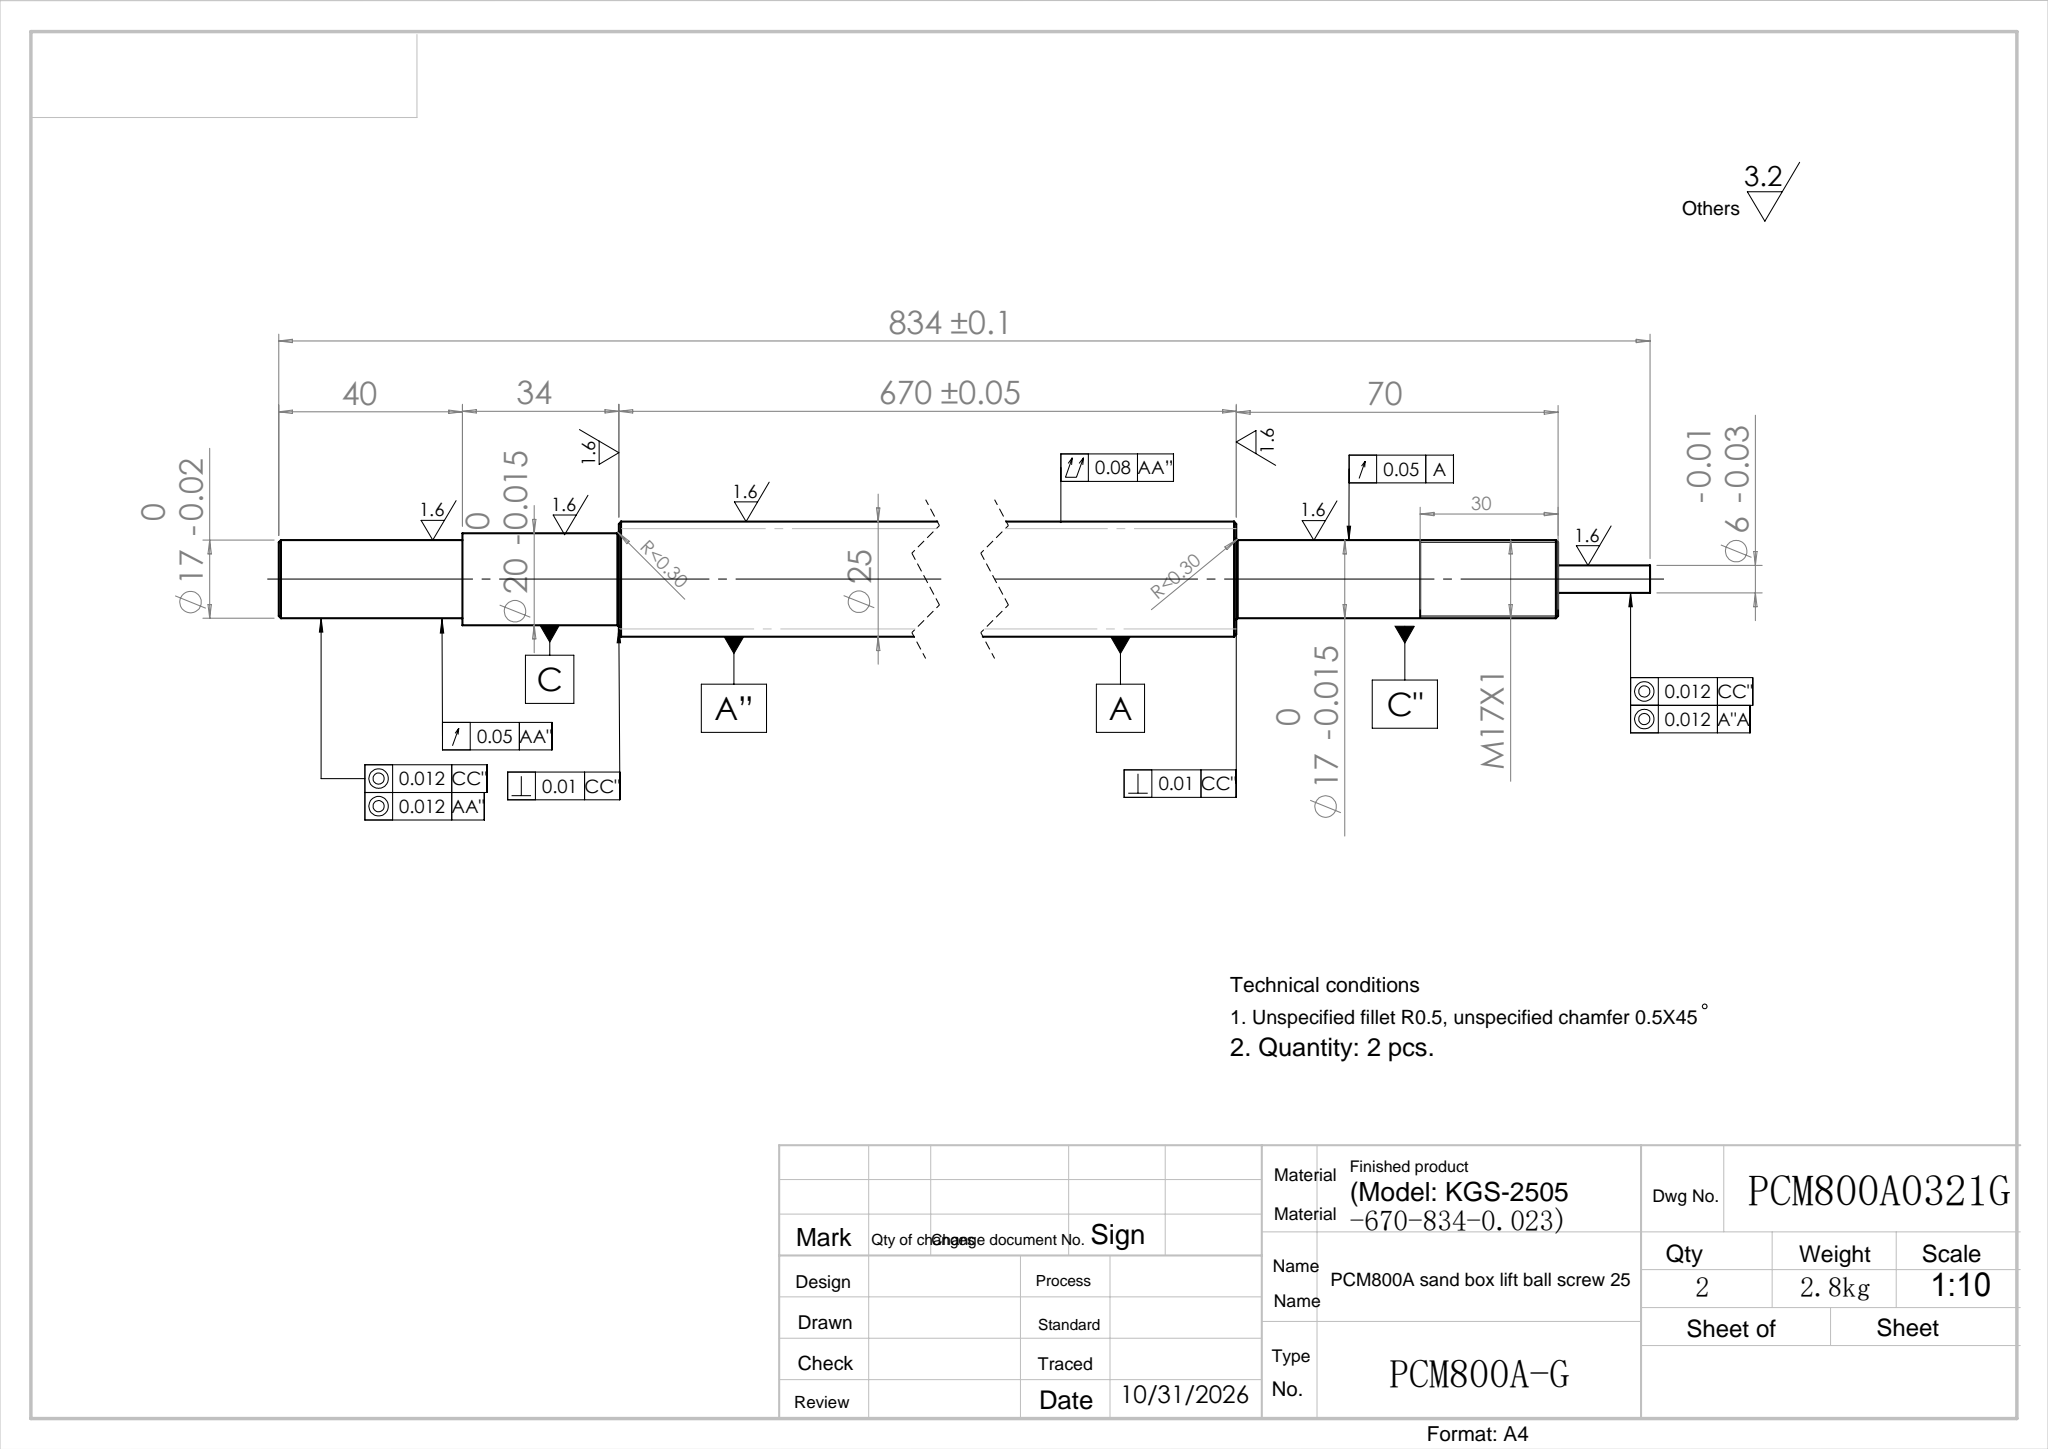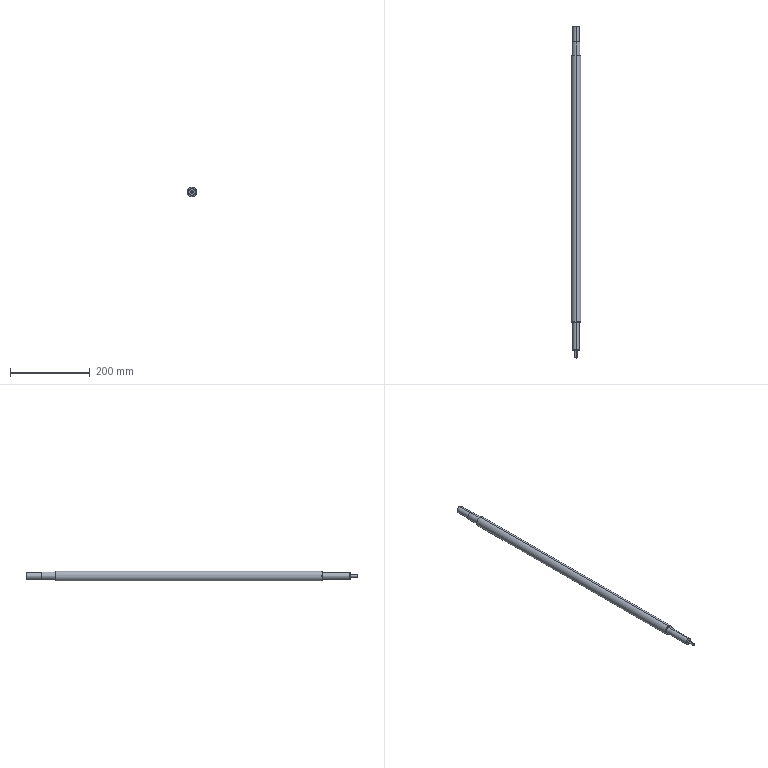Part | SolidWorks | features Boss 4, Fillet 2, Chamfer 1, Extrusion 1 | 1 solid | 28 faces | box 25 x 834 x 25 mm | volume 365070 mm3 | cylinder 10 | cone 8 | plane 6 | torus 4 | commonest cylinder face diameters 17 x4 6 x2 20 x2 25 x2
STEP:
#1=CARTESIAN_POINT('',(0.,-20.,-3.));
#2=VERTEX_POINT('',#1);
#3=CARTESIAN_POINT('',(0.,-20.,3.));
#4=VERTEX_POINT('',#3);
#5=CARTESIAN_POINT('',(0.,-20.,0.));
#6=DIRECTION('',(0.,-1.,0.));
#7=DIRECTION('',(0.,0.,-1.));
#8=AXIS2_PLACEMENT_3D('',#5,#6,#7);
#9=CIRCLE('',#8,3.);
#10=EDGE_CURVE('',#2,#4,#9,.T.);
#11=ORIENTED_EDGE('',*,*,#10,.F.);
#12=CARTESIAN_POINT('',(0.,0.,-3.));
#13=VERTEX_POINT('',#12);
#14=CARTESIAN_POINT('',(0.,-20.,-3.));
#15=DIRECTION('',(0.,1.,0.));
#16=VECTOR('',#15,1000.);
#17=LINE('',#14,#16);
#18=EDGE_CURVE('',#2,#13,#17,.T.);
#19=ORIENTED_EDGE('',*,*,#18,.T.);
#20=CARTESIAN_POINT('',(0.,0.,3.));
#21=VERTEX_POINT('',#20);
#22=CARTESIAN_POINT('',(0.,0.,0.));
#23=DIRECTION('',(0.,-1.,0.));
#24=DIRECTION('',(0.,0.,1.));
#25=AXIS2_PLACEMENT_3D('',#22,#23,#24);
#26=CIRCLE('',#25,3.);
#27=EDGE_CURVE('',#13,#21,#26,.T.);
#28=ORIENTED_EDGE('',*,*,#27,.T.);
#29=CARTESIAN_POINT('',(0.,-20.,3.));
#30=DIRECTION('',(0.,1.,0.));
#31=VECTOR('',#30,1000.);
#32=LINE('',#29,#31);
#33=EDGE_CURVE('',#4,#21,#32,.T.);
#34=ORIENTED_EDGE('',*,*,#33,.F.);
#35=EDGE_LOOP('',(#11,#19,#28,#34));
#36=FACE_OUTER_BOUND('',#35,.T.);
#37=CARTESIAN_POINT('',(0.,-20.,0.));
#38=DIRECTION('',(0.,1.,0.));
#39=DIRECTION('',(0.,0.,1.));
#40=AXIS2_PLACEMENT_3D('',#37,#38,#39);
#41=CYLINDRICAL_SURFACE('',#40,3.);
#42=ADVANCED_FACE('',(#36),#41,.T.);
#43=CARTESIAN_POINT('',(0.,740.3,-10.));
#44=VERTEX_POINT('',#43);
#45=CARTESIAN_POINT('',(0.,740.3,10.));
#46=VERTEX_POINT('',#45);
#47=CARTESIAN_POINT('',(0.,740.3,0.));
#48=DIRECTION('',(0.,1.,0.));
#49=DIRECTION('',(0.,0.,1.));
#50=AXIS2_PLACEMENT_3D('',#47,#48,#49);
#51=CIRCLE('',#50,10.);
#52=EDGE_CURVE('',#44,#46,#51,.T.);
#53=ORIENTED_EDGE('',*,*,#52,.F.);
#54=CARTESIAN_POINT('',(0.,740.,-10.3));
#55=VERTEX_POINT('',#54);
#56=CARTESIAN_POINT('',(0.,740.3,-10.3));
#57=DIRECTION('',(1.,0.,0.));
#58=DIRECTION('',(0.,0.,-1.));
#59=AXIS2_PLACEMENT_3D('',#56,#57,#58);
#60=CIRCLE('',#59,0.3);
#61=EDGE_CURVE('',#44,#55,#60,.T.);
#62=ORIENTED_EDGE('',*,*,#61,.T.);
#63=CARTESIAN_POINT('',(0.,740.,10.3));
#64=VERTEX_POINT('',#63);
#65=CARTESIAN_POINT('',(0.,740.,0.));
#66=DIRECTION('',(0.,-1.,0.));
#67=DIRECTION('',(0.,0.,1.));
#68=AXIS2_PLACEMENT_3D('',#65,#66,#67);
#69=CIRCLE('',#68,10.3);
#70=EDGE_CURVE('',#64,#55,#69,.T.);
#71=ORIENTED_EDGE('',*,*,#70,.F.);
#72=CARTESIAN_POINT('',(0.,740.3,10.3));
#73=DIRECTION('',(-1.,0.,0.));
#74=DIRECTION('',(0.,0.,1.));
#75=AXIS2_PLACEMENT_3D('',#72,#73,#74);
#76=CIRCLE('',#75,0.3);
#77=EDGE_CURVE('',#46,#64,#76,.T.);
#78=ORIENTED_EDGE('',*,*,#77,.F.);
#79=EDGE_LOOP('',(#53,#62,#71,#78));
#80=FACE_OUTER_BOUND('',#79,.T.);
#81=CARTESIAN_POINT('',(0.,740.3,0.));
#82=DIRECTION('',(0.,1.,0.));
#83=DIRECTION('',(0.,0.,1.));
#84=AXIS2_PLACEMENT_3D('',#81,#82,#83);
#85=TOROIDAL_SURFACE('',#84,10.3,0.3);
#86=ADVANCED_FACE('',(#80),#85,.F.);
#87=CARTESIAN_POINT('',(0.,70.,-8.8));
#88=VERTEX_POINT('',#87);
#89=CARTESIAN_POINT('',(0.,70.,8.8));
#90=VERTEX_POINT('',#89);
#91=CARTESIAN_POINT('',(0.,70.,0.));
#92=DIRECTION('',(0.,1.,0.));
#93=DIRECTION('',(0.,0.,1.));
#94=AXIS2_PLACEMENT_3D('',#91,#92,#93);
#95=CIRCLE('',#94,8.8);
#96=EDGE_CURVE('',#88,#90,#95,.T.);
#97=ORIENTED_EDGE('',*,*,#96,.F.);
#98=CARTESIAN_POINT('',(0.,69.7,-8.5));
#99=VERTEX_POINT('',#98);
#100=CARTESIAN_POINT('',(0.,69.7,-8.8));
#101=DIRECTION('',(1.,0.,0.));
#102=DIRECTION('',(0.,0.,-1.));
#103=AXIS2_PLACEMENT_3D('',#100,#101,#102);
#104=CIRCLE('',#103,0.3);
#105=EDGE_CURVE('',#88,#99,#104,.T.);
#106=ORIENTED_EDGE('',*,*,#105,.T.);
#107=CARTESIAN_POINT('',(0.,69.7,8.5));
#108=VERTEX_POINT('',#107);
#109=CARTESIAN_POINT('',(0.,69.7,0.));
#110=DIRECTION('',(0.,-1.,0.));
#111=DIRECTION('',(0.,0.,1.));
#112=AXIS2_PLACEMENT_3D('',#109,#110,#111);
#113=CIRCLE('',#112,8.5);
#114=EDGE_CURVE('',#108,#99,#113,.T.);
#115=ORIENTED_EDGE('',*,*,#114,.F.);
#116=CARTESIAN_POINT('',(0.,69.7,8.8));
#117=DIRECTION('',(-1.,0.,0.));
#118=DIRECTION('',(0.,0.,1.));
#119=AXIS2_PLACEMENT_3D('',#116,#117,#118);
#120=CIRCLE('',#119,0.3);
#121=EDGE_CURVE('',#90,#108,#120,.T.);
#122=ORIENTED_EDGE('',*,*,#121,.F.);
#123=EDGE_LOOP('',(#97,#106,#115,#122));
#124=FACE_OUTER_BOUND('',#123,.T.);
#125=CARTESIAN_POINT('',(0.,69.7,0.));
#126=DIRECTION('',(0.,1.,0.));
#127=DIRECTION('',(0.,0.,1.));
#128=AXIS2_PLACEMENT_3D('',#125,#126,#127);
#129=TOROIDAL_SURFACE('',#128,8.8,0.3);
#130=ADVANCED_FACE('',(#124),#129,.F.);
#131=CARTESIAN_POINT('',(0.,814.,8.));
#132=VERTEX_POINT('',#131);
#133=CARTESIAN_POINT('',(0.,814.,-8.));
#134=VERTEX_POINT('',#133);
#135=CARTESIAN_POINT('',(0.,814.,0.));
#136=DIRECTION('',(0.,1.,0.));
#137=DIRECTION('',(0.,0.,1.));
#138=AXIS2_PLACEMENT_3D('',#135,#136,#137);
#139=CIRCLE('',#138,8.);
#140=EDGE_CURVE('',#132,#134,#139,.T.);
#141=ORIENTED_EDGE('',*,*,#140,.F.);
#142=CARTESIAN_POINT('',(0.,813.5,8.5));
#143=VERTEX_POINT('',#142);
#144=CARTESIAN_POINT('',(0.,814.,8.));
#145=DIRECTION('',(0.,-0.7071,0.7071));
#146=VECTOR('',#145,1000.);
#147=LINE('',#144,#146);
#148=EDGE_CURVE('',#132,#143,#147,.T.);
#149=ORIENTED_EDGE('',*,*,#148,.T.);
#150=CARTESIAN_POINT('',(0.,813.5,-8.5));
#151=VERTEX_POINT('',#150);
#152=CARTESIAN_POINT('',(0.,813.5,0.));
#153=DIRECTION('',(0.,-1.,0.));
#154=DIRECTION('',(0.,0.,1.));
#155=AXIS2_PLACEMENT_3D('',#152,#153,#154);
#156=CIRCLE('',#155,8.5);
#157=EDGE_CURVE('',#151,#143,#156,.T.);
#158=ORIENTED_EDGE('',*,*,#157,.F.);
#159=CARTESIAN_POINT('',(0.,814.,-8.));
#160=DIRECTION('',(0.,-0.7071,-0.7071));
#161=VECTOR('',#160,1000.);
#162=LINE('',#159,#161);
#163=EDGE_CURVE('',#134,#151,#162,.T.);
#164=ORIENTED_EDGE('',*,*,#163,.F.);
#165=EDGE_LOOP('',(#141,#149,#158,#164));
#166=FACE_OUTER_BOUND('',#165,.T.);
#167=CARTESIAN_POINT('',(0.,814.,0.));
#168=DIRECTION('',(0.,-1.,0.));
#169=DIRECTION('',(0.,0.,-1.));
#170=AXIS2_PLACEMENT_3D('',#167,#168,#169);
#171=CONICAL_SURFACE('',#170,8.,0.7854);
#172=ADVANCED_FACE('',(#166),#171,.T.);
#173=CARTESIAN_POINT('',(0.,740.,12.));
#174=VERTEX_POINT('',#173);
#175=CARTESIAN_POINT('',(0.,740.,-12.));
#176=VERTEX_POINT('',#175);
#177=CARTESIAN_POINT('',(0.,740.,0.));
#178=DIRECTION('',(0.,1.,0.));
#179=DIRECTION('',(0.,0.,1.));
#180=AXIS2_PLACEMENT_3D('',#177,#178,#179);
#181=CIRCLE('',#180,12.);
#182=EDGE_CURVE('',#174,#176,#181,.T.);
#183=ORIENTED_EDGE('',*,*,#182,.F.);
#184=CARTESIAN_POINT('',(0.,739.5,12.5));
#185=VERTEX_POINT('',#184);
#186=CARTESIAN_POINT('',(0.,740.,12.));
#187=DIRECTION('',(0.,-0.7071,0.7071));
#188=VECTOR('',#187,1000.);
#189=LINE('',#186,#188);
#190=EDGE_CURVE('',#174,#185,#189,.T.);
#191=ORIENTED_EDGE('',*,*,#190,.T.);
#192=CARTESIAN_POINT('',(0.,739.5,-12.5));
#193=VERTEX_POINT('',#192);
#194=CARTESIAN_POINT('',(0.,739.5,0.));
#195=DIRECTION('',(0.,-1.,0.));
#196=DIRECTION('',(0.,0.,1.));
#197=AXIS2_PLACEMENT_3D('',#194,#195,#196);
#198=CIRCLE('',#197,12.5);
#199=EDGE_CURVE('',#193,#185,#198,.T.);
#200=ORIENTED_EDGE('',*,*,#199,.F.);
#201=CARTESIAN_POINT('',(0.,740.,-12.));
#202=DIRECTION('',(0.,-0.7071,-0.7071));
#203=VECTOR('',#202,1000.);
#204=LINE('',#201,#203);
#205=EDGE_CURVE('',#176,#193,#204,.T.);
#206=ORIENTED_EDGE('',*,*,#205,.F.);
#207=EDGE_LOOP('',(#183,#191,#200,#206));
#208=FACE_OUTER_BOUND('',#207,.T.);
#209=CARTESIAN_POINT('',(0.,740.,0.));
#210=DIRECTION('',(0.,-1.,0.));
#211=DIRECTION('',(0.,0.,-1.));
#212=AXIS2_PLACEMENT_3D('',#209,#210,#211);
#213=CONICAL_SURFACE('',#212,12.,0.7854);
#214=ADVANCED_FACE('',(#208),#213,.T.);
#215=CARTESIAN_POINT('',(0.,70.,-12.));
#216=VERTEX_POINT('',#215);
#217=CARTESIAN_POINT('',(0.,70.,12.));
#218=VERTEX_POINT('',#217);
#219=CARTESIAN_POINT('',(0.,70.,0.));
#220=DIRECTION('',(0.,-1.,0.));
#221=DIRECTION('',(0.,0.,1.));
#222=AXIS2_PLACEMENT_3D('',#219,#220,#221);
#223=CIRCLE('',#222,12.);
#224=EDGE_CURVE('',#216,#218,#223,.T.);
#225=ORIENTED_EDGE('',*,*,#224,.F.);
#226=CARTESIAN_POINT('',(0.,70.5,-12.5));
#227=VERTEX_POINT('',#226);
#228=CARTESIAN_POINT('',(0.,70.5,-12.5));
#229=DIRECTION('',(0.,0.7071,-0.7071));
#230=VECTOR('',#229,1000.);
#231=LINE('',#228,#230);
#232=EDGE_CURVE('',#216,#227,#231,.T.);
#233=ORIENTED_EDGE('',*,*,#232,.T.);
#234=CARTESIAN_POINT('',(0.,70.5,12.5));
#235=VERTEX_POINT('',#234);
#236=CARTESIAN_POINT('',(0.,70.5,0.));
#237=DIRECTION('',(0.,1.,0.));
#238=DIRECTION('',(0.,0.,1.));
#239=AXIS2_PLACEMENT_3D('',#236,#237,#238);
#240=CIRCLE('',#239,12.5);
#241=EDGE_CURVE('',#235,#227,#240,.T.);
#242=ORIENTED_EDGE('',*,*,#241,.F.);
#243=CARTESIAN_POINT('',(0.,70.5,12.5));
#244=DIRECTION('',(0.,0.7071,0.7071));
#245=VECTOR('',#244,1000.);
#246=LINE('',#243,#245);
#247=EDGE_CURVE('',#218,#235,#246,.T.);
#248=ORIENTED_EDGE('',*,*,#247,.F.);
#249=EDGE_LOOP('',(#225,#233,#242,#248));
#250=FACE_OUTER_BOUND('',#249,.T.);
#251=CARTESIAN_POINT('',(0.,70.5,0.));
#252=DIRECTION('',(0.,1.,0.));
#253=DIRECTION('',(0.,0.,1.));
#254=AXIS2_PLACEMENT_3D('',#251,#252,#253);
#255=CONICAL_SURFACE('',#254,12.5,0.7854);
#256=ADVANCED_FACE('',(#250),#255,.T.);
#257=CARTESIAN_POINT('',(0.,0.,-8.));
#258=VERTEX_POINT('',#257);
#259=CARTESIAN_POINT('',(0.,0.,8.));
#260=VERTEX_POINT('',#259);
#261=CARTESIAN_POINT('',(0.,0.,0.));
#262=DIRECTION('',(0.,-1.,0.));
#263=DIRECTION('',(0.,0.,1.));
#264=AXIS2_PLACEMENT_3D('',#261,#262,#263);
#265=CIRCLE('',#264,8.);
#266=EDGE_CURVE('',#258,#260,#265,.T.);
#267=ORIENTED_EDGE('',*,*,#266,.F.);
#268=CARTESIAN_POINT('',(0.,0.5,-8.5));
#269=VERTEX_POINT('',#268);
#270=CARTESIAN_POINT('',(0.,0.5,-8.5));
#271=DIRECTION('',(0.,0.7071,-0.7071));
#272=VECTOR('',#271,1000.);
#273=LINE('',#270,#272);
#274=EDGE_CURVE('',#258,#269,#273,.T.);
#275=ORIENTED_EDGE('',*,*,#274,.T.);
#276=CARTESIAN_POINT('',(0.,0.5,8.5));
#277=VERTEX_POINT('',#276);
#278=CARTESIAN_POINT('',(0.,0.5,0.));
#279=DIRECTION('',(0.,1.,0.));
#280=DIRECTION('',(0.,0.,1.));
#281=AXIS2_PLACEMENT_3D('',#278,#279,#280);
#282=CIRCLE('',#281,8.5);
#283=EDGE_CURVE('',#277,#269,#282,.T.);
#284=ORIENTED_EDGE('',*,*,#283,.F.);
#285=CARTESIAN_POINT('',(0.,0.5,8.5));
#286=DIRECTION('',(0.,0.7071,0.7071));
#287=VECTOR('',#286,1000.);
#288=LINE('',#285,#287);
#289=EDGE_CURVE('',#260,#277,#288,.T.);
#290=ORIENTED_EDGE('',*,*,#289,.F.);
#291=EDGE_LOOP('',(#267,#275,#284,#290));
#292=FACE_OUTER_BOUND('',#291,.T.);
#293=CARTESIAN_POINT('',(0.,0.5,0.));
#294=DIRECTION('',(0.,1.,0.));
#295=DIRECTION('',(0.,0.,1.));
#296=AXIS2_PLACEMENT_3D('',#293,#294,#295);
#297=CONICAL_SURFACE('',#296,8.5,0.7854);
#298=ADVANCED_FACE('',(#292),#297,.T.);
#299=ORIENTED_EDGE('',*,*,#157,.T.);
#300=CARTESIAN_POINT('',(0.,774.,8.5));
#301=VERTEX_POINT('',#300);
#302=CARTESIAN_POINT('',(0.,814.,8.5));
#303=DIRECTION('',(0.,-1.,0.));
#304=VECTOR('',#303,1000.);
#305=LINE('',#302,#304);
#306=EDGE_CURVE('',#143,#301,#305,.T.);
#307=ORIENTED_EDGE('',*,*,#306,.T.);
#308=CARTESIAN_POINT('',(0.,774.,-8.5));
#309=VERTEX_POINT('',#308);
#310=CARTESIAN_POINT('',(0.,774.,0.));
#311=DIRECTION('',(0.,1.,0.));
#312=DIRECTION('',(0.,0.,1.));
#313=AXIS2_PLACEMENT_3D('',#310,#311,#312);
#314=CIRCLE('',#313,8.5);
#315=EDGE_CURVE('',#301,#309,#314,.T.);
#316=ORIENTED_EDGE('',*,*,#315,.T.);
#317=CARTESIAN_POINT('',(0.,814.,-8.5));
#318=DIRECTION('',(0.,-1.,0.));
#319=VECTOR('',#318,1000.);
#320=LINE('',#317,#319);
#321=EDGE_CURVE('',#151,#309,#320,.T.);
#322=ORIENTED_EDGE('',*,*,#321,.F.);
#323=EDGE_LOOP('',(#299,#307,#316,#322));
#324=FACE_OUTER_BOUND('',#323,.T.);
#325=CARTESIAN_POINT('',(0.,814.,0.));
#326=DIRECTION('',(0.,-1.,0.));
#327=DIRECTION('',(0.,0.,-1.));
#328=AXIS2_PLACEMENT_3D('',#325,#326,#327);
#329=CYLINDRICAL_SURFACE('',#328,8.5);
#330=ADVANCED_FACE('',(#324),#329,.T.);
#331=CARTESIAN_POINT('',(0.,774.,10.));
#332=VERTEX_POINT('',#331);
#333=CARTESIAN_POINT('',(0.,774.,-10.));
#334=VERTEX_POINT('',#333);
#335=CARTESIAN_POINT('',(0.,774.,0.));
#336=DIRECTION('',(0.,1.,0.));
#337=DIRECTION('',(0.,0.,1.));
#338=AXIS2_PLACEMENT_3D('',#335,#336,#337);
#339=CIRCLE('',#338,10.);
#340=EDGE_CURVE('',#332,#334,#339,.T.);
#341=ORIENTED_EDGE('',*,*,#340,.F.);
#342=CARTESIAN_POINT('',(0.,774.,10.));
#343=DIRECTION('',(0.,-1.,0.));
#344=VECTOR('',#343,1000.);
#345=LINE('',#342,#344);
#346=EDGE_CURVE('',#332,#46,#345,.T.);
#347=ORIENTED_EDGE('',*,*,#346,.T.);
#348=CARTESIAN_POINT('',(0.,740.3,0.));
#349=DIRECTION('',(0.,1.,0.));
#350=DIRECTION('',(0.,0.,1.));
#351=AXIS2_PLACEMENT_3D('',#348,#349,#350);
#352=CIRCLE('',#351,10.);
#353=EDGE_CURVE('',#46,#44,#352,.T.);
#354=ORIENTED_EDGE('',*,*,#353,.T.);
#355=CARTESIAN_POINT('',(0.,774.,-10.));
#356=DIRECTION('',(0.,-1.,0.));
#357=VECTOR('',#356,1000.);
#358=LINE('',#355,#357);
#359=EDGE_CURVE('',#334,#44,#358,.T.);
#360=ORIENTED_EDGE('',*,*,#359,.F.);
#361=EDGE_LOOP('',(#341,#347,#354,#360));
#362=FACE_OUTER_BOUND('',#361,.T.);
#363=CARTESIAN_POINT('',(0.,774.,0.));
#364=DIRECTION('',(0.,-1.,0.));
#365=DIRECTION('',(0.,0.,-1.));
#366=AXIS2_PLACEMENT_3D('',#363,#364,#365);
#367=CYLINDRICAL_SURFACE('',#366,10.);
#368=ADVANCED_FACE('',(#362),#367,.T.);
#369=ORIENTED_EDGE('',*,*,#199,.T.);
#370=CARTESIAN_POINT('',(0.,740.,12.5));
#371=DIRECTION('',(0.,-1.,0.));
#372=VECTOR('',#371,1000.);
#373=LINE('',#370,#372);
#374=EDGE_CURVE('',#185,#235,#373,.T.);
#375=ORIENTED_EDGE('',*,*,#374,.T.);
#376=ORIENTED_EDGE('',*,*,#241,.T.);
#377=CARTESIAN_POINT('',(0.,740.,-12.5));
#378=DIRECTION('',(0.,-1.,0.));
#379=VECTOR('',#378,1000.);
#380=LINE('',#377,#379);
#381=EDGE_CURVE('',#193,#227,#380,.T.);
#382=ORIENTED_EDGE('',*,*,#381,.F.);
#383=EDGE_LOOP('',(#369,#375,#376,#382));
#384=FACE_OUTER_BOUND('',#383,.T.);
#385=CARTESIAN_POINT('',(0.,740.,0.));
#386=DIRECTION('',(0.,-1.,0.));
#387=DIRECTION('',(0.,0.,-1.));
#388=AXIS2_PLACEMENT_3D('',#385,#386,#387);
#389=CYLINDRICAL_SURFACE('',#388,12.5);
#390=ADVANCED_FACE('',(#384),#389,.T.);
#391=CARTESIAN_POINT('',(0.,69.7,0.));
#392=DIRECTION('',(0.,-1.,0.));
#393=DIRECTION('',(0.,0.,1.));
#394=AXIS2_PLACEMENT_3D('',#391,#392,#393);
#395=CIRCLE('',#394,8.5);
#396=EDGE_CURVE('',#99,#108,#395,.T.);
#397=ORIENTED_EDGE('',*,*,#396,.T.);
#398=CARTESIAN_POINT('',(0.,70.,8.5));
#399=DIRECTION('',(0.,-1.,0.));
#400=VECTOR('',#399,1000.);
#401=LINE('',#398,#400);
#402=EDGE_CURVE('',#108,#277,#401,.T.);
#403=ORIENTED_EDGE('',*,*,#402,.T.);
#404=ORIENTED_EDGE('',*,*,#283,.T.);
#405=CARTESIAN_POINT('',(0.,70.,-8.5));
#406=DIRECTION('',(0.,-1.,0.));
#407=VECTOR('',#406,1000.);
#408=LINE('',#405,#407);
#409=EDGE_CURVE('',#99,#269,#408,.T.);
#410=ORIENTED_EDGE('',*,*,#409,.F.);
#411=EDGE_LOOP('',(#397,#403,#404,#410));
#412=FACE_OUTER_BOUND('',#411,.T.);
#413=CARTESIAN_POINT('',(0.,70.,0.));
#414=DIRECTION('',(0.,-1.,0.));
#415=DIRECTION('',(0.,0.,-1.));
#416=AXIS2_PLACEMENT_3D('',#413,#414,#415);
#417=CYLINDRICAL_SURFACE('',#416,8.5);
#418=ADVANCED_FACE('',(#412),#417,.T.);
#419=CARTESIAN_POINT('',(0.,0.,0.));
#420=DIRECTION('',(0.,-1.,0.));
#421=DIRECTION('',(0.,0.,1.));
#422=AXIS2_PLACEMENT_3D('',#419,#420,#421);
#423=CIRCLE('',#422,8.);
#424=EDGE_CURVE('',#260,#258,#423,.T.);
#425=ORIENTED_EDGE('',*,*,#424,.T.);
#426=ORIENTED_EDGE('',*,*,#266,.T.);
#427=EDGE_LOOP('',(#425,#426));
#428=FACE_OUTER_BOUND('',#427,.T.);
#429=CARTESIAN_POINT('',(0.,0.,0.));
#430=DIRECTION('',(0.,-1.,0.));
#431=DIRECTION('',(0.,0.,1.));
#432=AXIS2_PLACEMENT_3D('',#429,#430,#431);
#433=CIRCLE('',#432,3.);
#434=EDGE_CURVE('',#21,#13,#433,.T.);
#435=ORIENTED_EDGE('',*,*,#434,.F.);
#436=ORIENTED_EDGE('',*,*,#27,.F.);
#437=EDGE_LOOP('',(#435,#436));
#438=FACE_BOUND('',#437,.T.);
#439=CARTESIAN_POINT('',(0.,0.,0.));
#440=DIRECTION('',(0.,1.,0.));
#441=DIRECTION('',(0.,0.,1.));
#442=AXIS2_PLACEMENT_3D('',#439,#440,#441);
#443=PLANE('',#442);
#444=ADVANCED_FACE('',(#428,#438),#443,.F.);
#445=CARTESIAN_POINT('',(0.,774.,0.));
#446=DIRECTION('',(0.,1.,0.));
#447=DIRECTION('',(0.,0.,1.));
#448=AXIS2_PLACEMENT_3D('',#445,#446,#447);
#449=CIRCLE('',#448,10.);
#450=EDGE_CURVE('',#334,#332,#449,.T.);
#451=ORIENTED_EDGE('',*,*,#450,.T.);
#452=ORIENTED_EDGE('',*,*,#340,.T.);
#453=EDGE_LOOP('',(#451,#452));
#454=FACE_OUTER_BOUND('',#453,.T.);
#455=CARTESIAN_POINT('',(0.,774.,0.));
#456=DIRECTION('',(0.,1.,0.));
#457=DIRECTION('',(0.,0.,1.));
#458=AXIS2_PLACEMENT_3D('',#455,#456,#457);
#459=CIRCLE('',#458,8.5);
#460=EDGE_CURVE('',#309,#301,#459,.T.);
#461=ORIENTED_EDGE('',*,*,#460,.F.);
#462=ORIENTED_EDGE('',*,*,#315,.F.);
#463=EDGE_LOOP('',(#461,#462));
#464=FACE_BOUND('',#463,.T.);
#465=CARTESIAN_POINT('',(0.,774.,0.));
#466=DIRECTION('',(0.,1.,0.));
#467=DIRECTION('',(0.,0.,1.));
#468=AXIS2_PLACEMENT_3D('',#465,#466,#467);
#469=PLANE('',#468);
#470=ADVANCED_FACE('',(#454,#464),#469,.T.);
#471=ORIENTED_EDGE('',*,*,#70,.T.);
#472=CARTESIAN_POINT('',(0.,740.,0.));
#473=DIRECTION('',(0.,-1.,0.));
#474=DIRECTION('',(0.,0.,1.));
#475=AXIS2_PLACEMENT_3D('',#472,#473,#474);
#476=CIRCLE('',#475,10.3);
#477=EDGE_CURVE('',#55,#64,#476,.T.);
#478=ORIENTED_EDGE('',*,*,#477,.T.);
#479=EDGE_LOOP('',(#471,#478));
#480=FACE_BOUND('',#479,.T.);
#481=CARTESIAN_POINT('',(0.,740.,0.));
#482=DIRECTION('',(0.,1.,0.));
#483=DIRECTION('',(0.,0.,1.));
#484=AXIS2_PLACEMENT_3D('',#481,#482,#483);
#485=CIRCLE('',#484,12.);
#486=EDGE_CURVE('',#176,#174,#485,.T.);
#487=ORIENTED_EDGE('',*,*,#486,.T.);
#488=ORIENTED_EDGE('',*,*,#182,.T.);
#489=EDGE_LOOP('',(#487,#488));
#490=FACE_OUTER_BOUND('',#489,.T.);
#491=CARTESIAN_POINT('',(0.,740.,0.));
#492=DIRECTION('',(0.,1.,0.));
#493=DIRECTION('',(0.,0.,1.));
#494=AXIS2_PLACEMENT_3D('',#491,#492,#493);
#495=PLANE('',#494);
#496=ADVANCED_FACE('',(#480,#490),#495,.T.);
#497=ORIENTED_EDGE('',*,*,#402,.F.);
#498=ORIENTED_EDGE('',*,*,#114,.T.);
#499=ORIENTED_EDGE('',*,*,#409,.T.);
#500=CARTESIAN_POINT('',(0.,0.5,0.));
#501=DIRECTION('',(0.,1.,0.));
#502=DIRECTION('',(0.,0.,1.));
#503=AXIS2_PLACEMENT_3D('',#500,#501,#502);
#504=CIRCLE('',#503,8.5);
#505=EDGE_CURVE('',#269,#277,#504,.T.);
#506=ORIENTED_EDGE('',*,*,#505,.T.);
#507=EDGE_LOOP('',(#497,#498,#499,#506));
#508=FACE_OUTER_BOUND('',#507,.T.);
#509=CARTESIAN_POINT('',(0.,70.,0.));
#510=DIRECTION('',(0.,-1.,0.));
#511=DIRECTION('',(0.,0.,-1.));
#512=AXIS2_PLACEMENT_3D('',#509,#510,#511);
#513=CYLINDRICAL_SURFACE('',#512,8.5);
#514=ADVANCED_FACE('',(#508),#513,.T.);
#515=CARTESIAN_POINT('',(0.,70.,0.));
#516=DIRECTION('',(0.,1.,0.));
#517=DIRECTION('',(0.,0.,1.));
#518=AXIS2_PLACEMENT_3D('',#515,#516,#517);
#519=CIRCLE('',#518,8.8);
#520=EDGE_CURVE('',#90,#88,#519,.T.);
#521=ORIENTED_EDGE('',*,*,#520,.T.);
#522=ORIENTED_EDGE('',*,*,#96,.T.);
#523=EDGE_LOOP('',(#521,#522));
#524=FACE_BOUND('',#523,.T.);
#525=CARTESIAN_POINT('',(0.,70.,0.));
#526=DIRECTION('',(0.,-1.,0.));
#527=DIRECTION('',(0.,0.,1.));
#528=AXIS2_PLACEMENT_3D('',#525,#526,#527);
#529=CIRCLE('',#528,12.);
#530=EDGE_CURVE('',#218,#216,#529,.T.);
#531=ORIENTED_EDGE('',*,*,#530,.T.);
#532=ORIENTED_EDGE('',*,*,#224,.T.);
#533=EDGE_LOOP('',(#531,#532));
#534=FACE_OUTER_BOUND('',#533,.T.);
#535=CARTESIAN_POINT('',(0.,70.,0.));
#536=DIRECTION('',(0.,1.,0.));
#537=DIRECTION('',(0.,0.,1.));
#538=AXIS2_PLACEMENT_3D('',#535,#536,#537);
#539=PLANE('',#538);
#540=ADVANCED_FACE('',(#524,#534),#539,.F.);
#541=ORIENTED_EDGE('',*,*,#374,.F.);
#542=CARTESIAN_POINT('',(0.,739.5,0.));
#543=DIRECTION('',(0.,-1.,0.));
#544=DIRECTION('',(0.,0.,1.));
#545=AXIS2_PLACEMENT_3D('',#542,#543,#544);
#546=CIRCLE('',#545,12.5);
#547=EDGE_CURVE('',#185,#193,#546,.T.);
#548=ORIENTED_EDGE('',*,*,#547,.T.);
#549=ORIENTED_EDGE('',*,*,#381,.T.);
#550=CARTESIAN_POINT('',(0.,70.5,0.));
#551=DIRECTION('',(0.,1.,0.));
#552=DIRECTION('',(0.,0.,1.));
#553=AXIS2_PLACEMENT_3D('',#550,#551,#552);
#554=CIRCLE('',#553,12.5);
#555=EDGE_CURVE('',#227,#235,#554,.T.);
#556=ORIENTED_EDGE('',*,*,#555,.T.);
#557=EDGE_LOOP('',(#541,#548,#549,#556));
#558=FACE_OUTER_BOUND('',#557,.T.);
#559=CARTESIAN_POINT('',(0.,740.,0.));
#560=DIRECTION('',(0.,-1.,0.));
#561=DIRECTION('',(0.,0.,-1.));
#562=AXIS2_PLACEMENT_3D('',#559,#560,#561);
#563=CYLINDRICAL_SURFACE('',#562,12.5);
#564=ADVANCED_FACE('',(#558),#563,.T.);
#565=ORIENTED_EDGE('',*,*,#346,.F.);
#566=ORIENTED_EDGE('',*,*,#450,.F.);
#567=ORIENTED_EDGE('',*,*,#359,.T.);
#568=ORIENTED_EDGE('',*,*,#52,.T.);
#569=EDGE_LOOP('',(#565,#566,#567,#568));
#570=FACE_OUTER_BOUND('',#569,.T.);
#571=CARTESIAN_POINT('',(0.,774.,0.));
#572=DIRECTION('',(0.,-1.,0.));
#573=DIRECTION('',(0.,0.,-1.));
#574=AXIS2_PLACEMENT_3D('',#571,#572,#573);
#575=CYLINDRICAL_SURFACE('',#574,10.);
#576=ADVANCED_FACE('',(#570),#575,.T.);
#577=ORIENTED_EDGE('',*,*,#306,.F.);
#578=CARTESIAN_POINT('',(0.,813.5,0.));
#579=DIRECTION('',(0.,-1.,0.));
#580=DIRECTION('',(0.,0.,1.));
#581=AXIS2_PLACEMENT_3D('',#578,#579,#580);
#582=CIRCLE('',#581,8.5);
#583=EDGE_CURVE('',#143,#151,#582,.T.);
#584=ORIENTED_EDGE('',*,*,#583,.T.);
#585=ORIENTED_EDGE('',*,*,#321,.T.);
#586=ORIENTED_EDGE('',*,*,#460,.T.);
#587=EDGE_LOOP('',(#577,#584,#585,#586));
#588=FACE_OUTER_BOUND('',#587,.T.);
#589=CARTESIAN_POINT('',(0.,814.,0.));
#590=DIRECTION('',(0.,-1.,0.));
#591=DIRECTION('',(0.,0.,-1.));
#592=AXIS2_PLACEMENT_3D('',#589,#590,#591);
#593=CYLINDRICAL_SURFACE('',#592,8.5);
#594=ADVANCED_FACE('',(#588),#593,.T.);
#595=CARTESIAN_POINT('',(0.,814.,0.));
#596=DIRECTION('',(0.,1.,0.));
#597=DIRECTION('',(0.,0.,1.));
#598=AXIS2_PLACEMENT_3D('',#595,#596,#597);
#599=CIRCLE('',#598,8.);
#600=EDGE_CURVE('',#134,#132,#599,.T.);
#601=ORIENTED_EDGE('',*,*,#600,.T.);
#602=ORIENTED_EDGE('',*,*,#140,.T.);
#603=EDGE_LOOP('',(#601,#602));
#604=FACE_OUTER_BOUND('',#603,.T.);
#605=CARTESIAN_POINT('',(0.,814.,0.));
#606=DIRECTION('',(0.,1.,0.));
#607=DIRECTION('',(0.,0.,1.));
#608=AXIS2_PLACEMENT_3D('',#605,#606,#607);
#609=PLANE('',#608);
#610=ADVANCED_FACE('',(#604),#609,.T.);
#611=ORIENTED_EDGE('',*,*,#274,.F.);
#612=ORIENTED_EDGE('',*,*,#424,.F.);
#613=ORIENTED_EDGE('',*,*,#289,.T.);
#614=ORIENTED_EDGE('',*,*,#505,.F.);
#615=EDGE_LOOP('',(#611,#612,#613,#614));
#616=FACE_OUTER_BOUND('',#615,.T.);
#617=CARTESIAN_POINT('',(0.,0.5,0.));
#618=DIRECTION('',(0.,1.,0.));
#619=DIRECTION('',(0.,0.,1.));
#620=AXIS2_PLACEMENT_3D('',#617,#618,#619);
#621=CONICAL_SURFACE('',#620,8.5,0.7854);
#622=ADVANCED_FACE('',(#616),#621,.T.);
#623=ORIENTED_EDGE('',*,*,#232,.F.);
#624=ORIENTED_EDGE('',*,*,#530,.F.);
#625=ORIENTED_EDGE('',*,*,#247,.T.);
#626=ORIENTED_EDGE('',*,*,#555,.F.);
#627=EDGE_LOOP('',(#623,#624,#625,#626));
#628=FACE_OUTER_BOUND('',#627,.T.);
#629=CARTESIAN_POINT('',(0.,70.5,0.));
#630=DIRECTION('',(0.,1.,0.));
#631=DIRECTION('',(0.,0.,1.));
#632=AXIS2_PLACEMENT_3D('',#629,#630,#631);
#633=CONICAL_SURFACE('',#632,12.5,0.7854);
#634=ADVANCED_FACE('',(#628),#633,.T.);
#635=ORIENTED_EDGE('',*,*,#190,.F.);
#636=ORIENTED_EDGE('',*,*,#486,.F.);
#637=ORIENTED_EDGE('',*,*,#205,.T.);
#638=ORIENTED_EDGE('',*,*,#547,.F.);
#639=EDGE_LOOP('',(#635,#636,#637,#638));
#640=FACE_OUTER_BOUND('',#639,.T.);
#641=CARTESIAN_POINT('',(0.,740.,0.));
#642=DIRECTION('',(0.,-1.,0.));
#643=DIRECTION('',(0.,0.,-1.));
#644=AXIS2_PLACEMENT_3D('',#641,#642,#643);
#645=CONICAL_SURFACE('',#644,12.,0.7854);
#646=ADVANCED_FACE('',(#640),#645,.T.);
#647=ORIENTED_EDGE('',*,*,#148,.F.);
#648=ORIENTED_EDGE('',*,*,#600,.F.);
#649=ORIENTED_EDGE('',*,*,#163,.T.);
#650=ORIENTED_EDGE('',*,*,#583,.F.);
#651=EDGE_LOOP('',(#647,#648,#649,#650));
#652=FACE_OUTER_BOUND('',#651,.T.);
#653=CARTESIAN_POINT('',(0.,814.,0.));
#654=DIRECTION('',(0.,-1.,0.));
#655=DIRECTION('',(0.,0.,-1.));
#656=AXIS2_PLACEMENT_3D('',#653,#654,#655);
#657=CONICAL_SURFACE('',#656,8.,0.7854);
#658=ADVANCED_FACE('',(#652),#657,.T.);
#659=ORIENTED_EDGE('',*,*,#105,.F.);
#660=ORIENTED_EDGE('',*,*,#520,.F.);
#661=ORIENTED_EDGE('',*,*,#121,.T.);
#662=ORIENTED_EDGE('',*,*,#396,.F.);
#663=EDGE_LOOP('',(#659,#660,#661,#662));
#664=FACE_OUTER_BOUND('',#663,.T.);
#665=CARTESIAN_POINT('',(0.,69.7,0.));
#666=DIRECTION('',(0.,1.,0.));
#667=DIRECTION('',(0.,0.,1.));
#668=AXIS2_PLACEMENT_3D('',#665,#666,#667);
#669=TOROIDAL_SURFACE('',#668,8.8,0.3);
#670=ADVANCED_FACE('',(#664),#669,.F.);
#671=ORIENTED_EDGE('',*,*,#61,.F.);
#672=ORIENTED_EDGE('',*,*,#353,.F.);
#673=ORIENTED_EDGE('',*,*,#77,.T.);
#674=ORIENTED_EDGE('',*,*,#477,.F.);
#675=EDGE_LOOP('',(#671,#672,#673,#674));
#676=FACE_OUTER_BOUND('',#675,.T.);
#677=CARTESIAN_POINT('',(0.,740.3,0.));
#678=DIRECTION('',(0.,1.,0.));
#679=DIRECTION('',(0.,0.,1.));
#680=AXIS2_PLACEMENT_3D('',#677,#678,#679);
#681=TOROIDAL_SURFACE('',#680,10.3,0.3);
#682=ADVANCED_FACE('',(#676),#681,.F.);
#683=ORIENTED_EDGE('',*,*,#18,.F.);
#684=CARTESIAN_POINT('',(0.,-20.,0.));
#685=DIRECTION('',(0.,-1.,0.));
#686=DIRECTION('',(0.,0.,-1.));
#687=AXIS2_PLACEMENT_3D('',#684,#685,#686);
#688=CIRCLE('',#687,3.);
#689=EDGE_CURVE('',#4,#2,#688,.T.);
#690=ORIENTED_EDGE('',*,*,#689,.F.);
#691=ORIENTED_EDGE('',*,*,#33,.T.);
#692=ORIENTED_EDGE('',*,*,#434,.T.);
#693=EDGE_LOOP('',(#683,#690,#691,#692));
#694=FACE_OUTER_BOUND('',#693,.T.);
#695=CARTESIAN_POINT('',(0.,-20.,0.));
#696=DIRECTION('',(0.,1.,0.));
#697=DIRECTION('',(0.,0.,1.));
#698=AXIS2_PLACEMENT_3D('',#695,#696,#697);
#699=CYLINDRICAL_SURFACE('',#698,3.);
#700=ADVANCED_FACE('',(#694),#699,.T.);
#701=ORIENTED_EDGE('',*,*,#689,.T.);
#702=ORIENTED_EDGE('',*,*,#10,.T.);
#703=EDGE_LOOP('',(#701,#702));
#704=FACE_OUTER_BOUND('',#703,.T.);
#705=CARTESIAN_POINT('',(0.,-20.,0.));
#706=DIRECTION('',(0.,-1.,0.));
#707=DIRECTION('',(0.,0.,-1.));
#708=AXIS2_PLACEMENT_3D('',#705,#706,#707);
#709=PLANE('',#708);
#710=ADVANCED_FACE('',(#704),#709,.T.);
#711=CLOSED_SHELL('',(#42,#86,#130,#172,#214,#256,#298,#330,#368,#390,#418,#444,#470,#496,#514,#540,#564,#576,#594,#610,#622,#634,#646,#658,#670,#682,#700,#710));
#712=MANIFOLD_SOLID_BREP('',#711);
#713=CARTESIAN_POINT('',(0.,0.,0.));
#714=DIRECTION('',(0.,0.,1.));
#715=DIRECTION('',(1.,0.,0.));
#716=AXIS2_PLACEMENT_3D('',#713,#714,#715);
#717=(LENGTH_UNIT()NAMED_UNIT(*)SI_UNIT(.MILLI.,.METRE.));
#718=UNCERTAINTY_MEASURE_WITH_UNIT(LENGTH_MEASURE(0.00001),#717,'','');
#719=(NAMED_UNIT(*)PLANE_ANGLE_UNIT()SI_UNIT($,.RADIAN.));
#720=(NAMED_UNIT(*)SI_UNIT($,.STERADIAN.)SOLID_ANGLE_UNIT());
#721=(GEOMETRIC_REPRESENTATION_CONTEXT(3)GLOBAL_UNCERTAINTY_ASSIGNED_CONTEXT((#718))GLOBAL_UNIT_ASSIGNED_CONTEXT((#717,#719,#720))REPRESENTATION_CONTEXT('',''));
#722=ADVANCED_BREP_SHAPE_REPRESENTATION('',(#712,#716),#721);